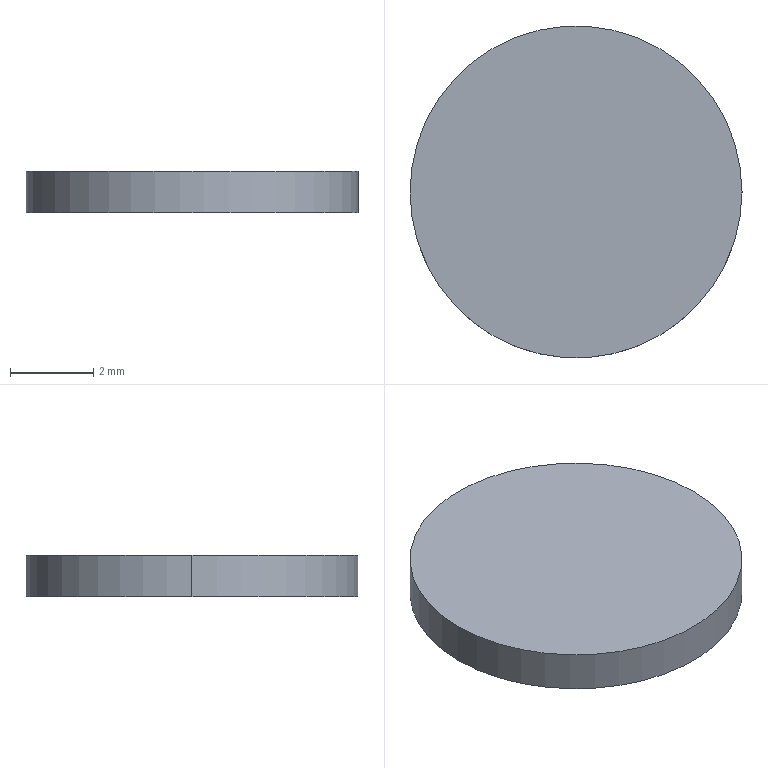Part | STEP file | 1 solid | 4 faces | box 8 x 8 x 1 mm | volume 50.265 mm3 | plane 2 | cylinder 2 | commonest cylinder face diameters 8 x2
STEP:
#1=CARTESIAN_POINT('',(0.,0.,0.));
#2=DIRECTION('',(0.,0.,1.));
#3=DIRECTION('',(1.,0.,0.));
#4=AXIS2_PLACEMENT_3D('',#1,#2,#3);
#5=CARTESIAN_POINT('',(-4.,0.,0.));
#6=VERTEX_POINT('',#5);
#7=CARTESIAN_POINT('',(4.,0.,0.));
#8=VERTEX_POINT('',#7);
#9=CARTESIAN_POINT('',(0.,0.,0.));
#10=DIRECTION('',(0.,0.,1.));
#11=DIRECTION('',(1.,0.,0.));
#12=AXIS2_PLACEMENT_3D('',#9,#10,#11);
#13=CIRCLE('',#12,4.);
#14=CARTESIAN_POINT('',(0.,0.,0.));
#15=DIRECTION('',(0.,0.,1.));
#16=DIRECTION('',(1.,0.,0.));
#17=AXIS2_PLACEMENT_3D('',#14,#15,#16);
#18=PLANE('',#17);
#19=CARTESIAN_POINT('',(0.,0.));
#20=DIRECTION('',(1.,0.));
#21=AXIS2_PLACEMENT_2D('',#19,#20);
#22=CIRCLE('',#21,4.);
#23=(GEOMETRIC_REPRESENTATION_CONTEXT(2)PARAMETRIC_REPRESENTATION_CONTEXT()REPRESENTATION_CONTEXT('',''));
#24=DEFINITIONAL_REPRESENTATION('',(#22),#23);
#25=PCURVE('',#18,#24);
#26=CARTESIAN_POINT('',(0.,0.,1.));
#27=DIRECTION('',(0.,0.,-1.));
#28=DIRECTION('',(-1.,0.,0.));
#29=AXIS2_PLACEMENT_3D('',#26,#27,#28);
#30=CYLINDRICAL_SURFACE('',#29,4.);
#31=CARTESIAN_POINT('',(9.425,1.));
#32=DIRECTION('',(-1.,0.));
#33=VECTOR('',#32,1.);
#34=LINE('',#31,#33);
#35=(GEOMETRIC_REPRESENTATION_CONTEXT(2)PARAMETRIC_REPRESENTATION_CONTEXT()REPRESENTATION_CONTEXT('',''));
#36=DEFINITIONAL_REPRESENTATION('',(#34),#35);
#37=PCURVE('',#30,#36);
#38=SURFACE_CURVE('',#13,(#25,#37),.PCURVE_S1.);
#39=EDGE_CURVE('',#6,#8,#38,.T.);
#40=ORIENTED_EDGE('',*,*,#39,.F.);
#41=CARTESIAN_POINT('',(0.,0.,0.));
#42=DIRECTION('',(0.,0.,1.));
#43=DIRECTION('',(1.,0.,0.));
#44=AXIS2_PLACEMENT_3D('',#41,#42,#43);
#45=CIRCLE('',#44,4.);
#46=CARTESIAN_POINT('',(0.,0.));
#47=DIRECTION('',(1.,0.));
#48=AXIS2_PLACEMENT_2D('',#46,#47);
#49=CIRCLE('',#48,4.);
#50=(GEOMETRIC_REPRESENTATION_CONTEXT(2)PARAMETRIC_REPRESENTATION_CONTEXT()REPRESENTATION_CONTEXT('',''));
#51=DEFINITIONAL_REPRESENTATION('',(#49),#50);
#52=PCURVE('',#18,#51);
#53=CARTESIAN_POINT('',(0.,0.,1.));
#54=DIRECTION('',(0.,0.,-1.));
#55=DIRECTION('',(-1.,0.,0.));
#56=AXIS2_PLACEMENT_3D('',#53,#54,#55);
#57=CYLINDRICAL_SURFACE('',#56,4.);
#58=CARTESIAN_POINT('',(3.142,1.));
#59=DIRECTION('',(-1.,0.));
#60=VECTOR('',#59,1.);
#61=LINE('',#58,#60);
#62=(GEOMETRIC_REPRESENTATION_CONTEXT(2)PARAMETRIC_REPRESENTATION_CONTEXT()REPRESENTATION_CONTEXT('',''));
#63=DEFINITIONAL_REPRESENTATION('',(#61),#62);
#64=PCURVE('',#57,#63);
#65=SURFACE_CURVE('',#45,(#52,#64),.PCURVE_S1.);
#66=EDGE_CURVE('',#8,#6,#65,.T.);
#67=ORIENTED_EDGE('',*,*,#66,.F.);
#68=EDGE_LOOP('',(#40,#67));
#69=FACE_BOUND('',#68,.T.);
#70=ADVANCED_FACE('',(#69),#18,.F.);
#71=CARTESIAN_POINT('',(-4.,0.,1.));
#72=VERTEX_POINT('',#71);
#73=CARTESIAN_POINT('',(4.,0.,1.));
#74=VERTEX_POINT('',#73);
#75=CARTESIAN_POINT('',(0.,0.,1.));
#76=DIRECTION('',(0.,0.,1.));
#77=DIRECTION('',(1.,0.,0.));
#78=AXIS2_PLACEMENT_3D('',#75,#76,#77);
#79=CIRCLE('',#78,4.);
#80=CARTESIAN_POINT('',(0.,0.,1.));
#81=DIRECTION('',(0.,0.,1.));
#82=DIRECTION('',(1.,0.,0.));
#83=AXIS2_PLACEMENT_3D('',#80,#81,#82);
#84=PLANE('',#83);
#85=CARTESIAN_POINT('',(0.,0.));
#86=DIRECTION('',(1.,0.));
#87=AXIS2_PLACEMENT_2D('',#85,#86);
#88=CIRCLE('',#87,4.);
#89=(GEOMETRIC_REPRESENTATION_CONTEXT(2)PARAMETRIC_REPRESENTATION_CONTEXT()REPRESENTATION_CONTEXT('',''));
#90=DEFINITIONAL_REPRESENTATION('',(#88),#89);
#91=PCURVE('',#84,#90);
#92=CARTESIAN_POINT('',(9.425,0.));
#93=DIRECTION('',(-1.,0.));
#94=VECTOR('',#93,1.);
#95=LINE('',#92,#94);
#96=(GEOMETRIC_REPRESENTATION_CONTEXT(2)PARAMETRIC_REPRESENTATION_CONTEXT()REPRESENTATION_CONTEXT('',''));
#97=DEFINITIONAL_REPRESENTATION('',(#95),#96);
#98=PCURVE('',#30,#97);
#99=SURFACE_CURVE('',#79,(#91,#98),.PCURVE_S1.);
#100=EDGE_CURVE('',#72,#74,#99,.T.);
#101=ORIENTED_EDGE('',*,*,#100,.T.);
#102=CARTESIAN_POINT('',(0.,0.,1.));
#103=DIRECTION('',(0.,0.,1.));
#104=DIRECTION('',(1.,0.,0.));
#105=AXIS2_PLACEMENT_3D('',#102,#103,#104);
#106=CIRCLE('',#105,4.);
#107=CARTESIAN_POINT('',(0.,0.));
#108=DIRECTION('',(1.,0.));
#109=AXIS2_PLACEMENT_2D('',#107,#108);
#110=CIRCLE('',#109,4.);
#111=(GEOMETRIC_REPRESENTATION_CONTEXT(2)PARAMETRIC_REPRESENTATION_CONTEXT()REPRESENTATION_CONTEXT('',''));
#112=DEFINITIONAL_REPRESENTATION('',(#110),#111);
#113=PCURVE('',#84,#112);
#114=CARTESIAN_POINT('',(3.142,0.));
#115=DIRECTION('',(-1.,0.));
#116=VECTOR('',#115,1.);
#117=LINE('',#114,#116);
#118=(GEOMETRIC_REPRESENTATION_CONTEXT(2)PARAMETRIC_REPRESENTATION_CONTEXT()REPRESENTATION_CONTEXT('',''));
#119=DEFINITIONAL_REPRESENTATION('',(#117),#118);
#120=PCURVE('',#57,#119);
#121=SURFACE_CURVE('',#106,(#113,#120),.PCURVE_S1.);
#122=EDGE_CURVE('',#74,#72,#121,.T.);
#123=ORIENTED_EDGE('',*,*,#122,.T.);
#124=EDGE_LOOP('',(#101,#123));
#125=FACE_BOUND('',#124,.T.);
#126=ADVANCED_FACE('',(#125),#84,.T.);
#127=CARTESIAN_POINT('',(4.,0.,1.));
#128=DIRECTION('',(0.,0.,-1.));
#129=VECTOR('',#128,1.);
#130=LINE('',#127,#129);
#131=CARTESIAN_POINT('',(3.142,0.));
#132=DIRECTION('',(0.,1.));
#133=VECTOR('',#132,1.);
#134=LINE('',#131,#133);
#135=(GEOMETRIC_REPRESENTATION_CONTEXT(2)PARAMETRIC_REPRESENTATION_CONTEXT()REPRESENTATION_CONTEXT('',''));
#136=DEFINITIONAL_REPRESENTATION('',(#134),#135);
#137=PCURVE('',#30,#136);
#138=CARTESIAN_POINT('',(3.142,0.));
#139=DIRECTION('',(0.,1.));
#140=VECTOR('',#139,1.);
#141=LINE('',#138,#140);
#142=(GEOMETRIC_REPRESENTATION_CONTEXT(2)PARAMETRIC_REPRESENTATION_CONTEXT()REPRESENTATION_CONTEXT('',''));
#143=DEFINITIONAL_REPRESENTATION('',(#141),#142);
#144=PCURVE('',#57,#143);
#145=SURFACE_CURVE('',#130,(#137,#144),.PCURVE_S1.);
#146=EDGE_CURVE('',#74,#8,#145,.T.);
#147=ORIENTED_EDGE('',*,*,#146,.F.);
#148=ORIENTED_EDGE('',*,*,#100,.F.);
#149=CARTESIAN_POINT('',(-4.,0.,1.));
#150=DIRECTION('',(0.,0.,-1.));
#151=VECTOR('',#150,1.);
#152=LINE('',#149,#151);
#153=CARTESIAN_POINT('',(6.283,0.));
#154=DIRECTION('',(0.,1.));
#155=VECTOR('',#154,1.);
#156=LINE('',#153,#155);
#157=(GEOMETRIC_REPRESENTATION_CONTEXT(2)PARAMETRIC_REPRESENTATION_CONTEXT()REPRESENTATION_CONTEXT('',''));
#158=DEFINITIONAL_REPRESENTATION('',(#156),#157);
#159=PCURVE('',#30,#158);
#160=CARTESIAN_POINT('',(0.,0.));
#161=DIRECTION('',(0.,1.));
#162=VECTOR('',#161,1.);
#163=LINE('',#160,#162);
#164=(GEOMETRIC_REPRESENTATION_CONTEXT(2)PARAMETRIC_REPRESENTATION_CONTEXT()REPRESENTATION_CONTEXT('',''));
#165=DEFINITIONAL_REPRESENTATION('',(#163),#164);
#166=PCURVE('',#57,#165);
#167=SURFACE_CURVE('',#152,(#159,#166),.PCURVE_S1.);
#168=EDGE_CURVE('',#72,#6,#167,.T.);
#169=ORIENTED_EDGE('',*,*,#168,.T.);
#170=ORIENTED_EDGE('',*,*,#39,.T.);
#171=EDGE_LOOP('',(#147,#148,#169,#170));
#172=FACE_BOUND('',#171,.T.);
#173=ADVANCED_FACE('',(#172),#30,.T.);
#174=ORIENTED_EDGE('',*,*,#122,.F.);
#175=ORIENTED_EDGE('',*,*,#146,.T.);
#176=ORIENTED_EDGE('',*,*,#66,.T.);
#177=ORIENTED_EDGE('',*,*,#168,.F.);
#178=EDGE_LOOP('',(#174,#175,#176,#177));
#179=FACE_BOUND('',#178,.T.);
#180=ADVANCED_FACE('',(#179),#57,.T.);
#181=CLOSED_SHELL('',(#70,#126,#173,#180));
#182=MANIFOLD_SOLID_BREP('',#181);
#183=(LENGTH_UNIT()NAMED_UNIT(*)SI_UNIT(.MILLI.,.METRE.));
#184=UNCERTAINTY_MEASURE_WITH_UNIT(LENGTH_MEASURE(0.0000001),#183,'','');
#185=(NAMED_UNIT(*)PLANE_ANGLE_UNIT()SI_UNIT($,.RADIAN.));
#186=(NAMED_UNIT(*)SI_UNIT($,.STERADIAN.)SOLID_ANGLE_UNIT());
#187=(GEOMETRIC_REPRESENTATION_CONTEXT(3)GLOBAL_UNCERTAINTY_ASSIGNED_CONTEXT((#184))GLOBAL_UNIT_ASSIGNED_CONTEXT((#183,#185,#186))REPRESENTATION_CONTEXT('',''));
#188=ADVANCED_BREP_SHAPE_REPRESENTATION('',(#4,#182),#187);